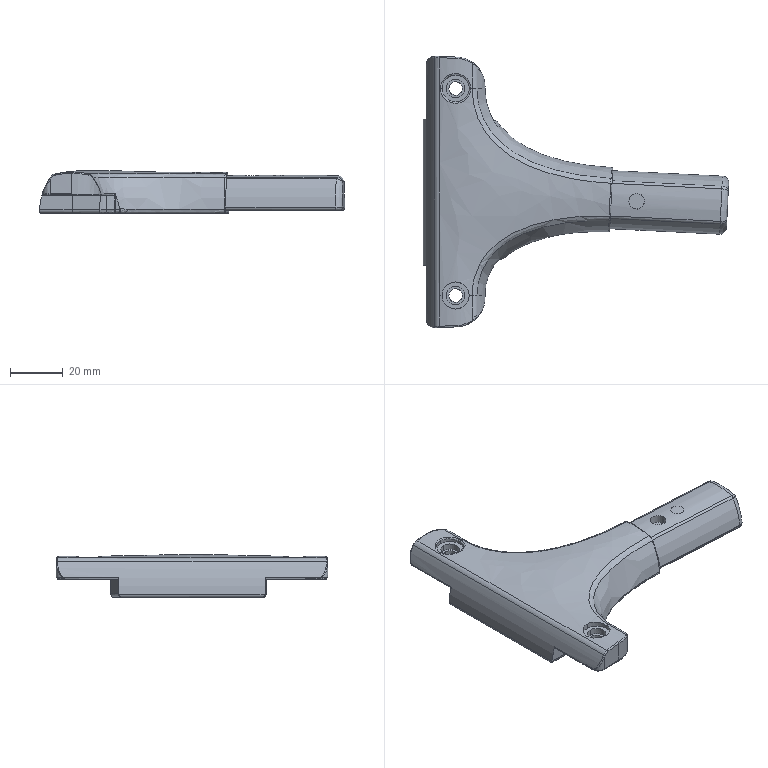Part | SolidWorks | features BaseBody 1 | 1 solid | 543 faces | box 115.648 x 102.814 x 16.383 mm | volume 42708 mm3 | plane 275 | spline 143 | cylinder 125 | commonest cylinder face diameters 2.745 x14 0.98 x11 5.882 x10 41.765 x10 2.941 x7 24.51 x7